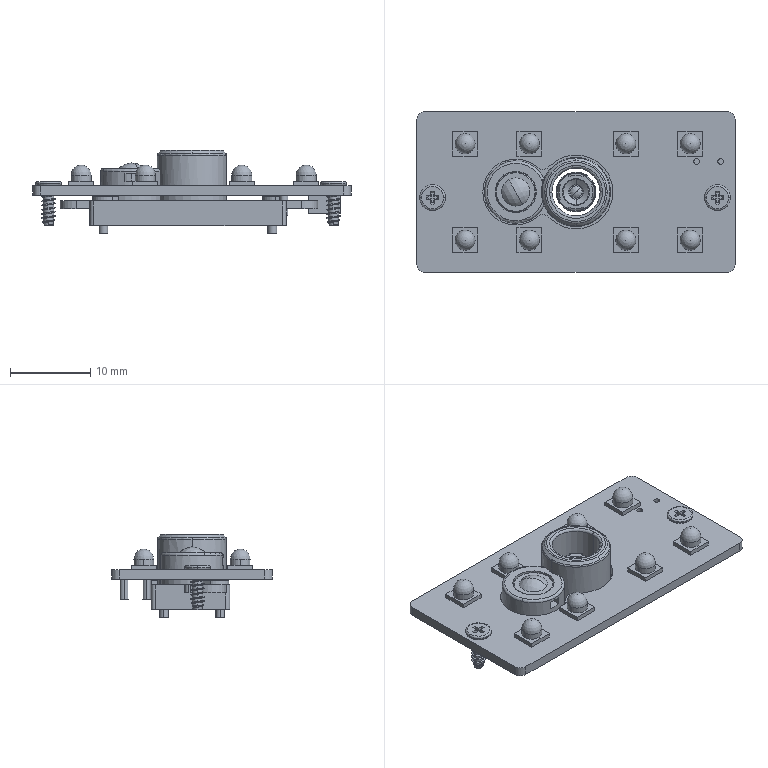Part | SolidWorks | 6 solids | 432 faces | box 39.6 x 20 x 10.4 mm | volume 1839 mm3 | cylinder 169 | plane 160 | cone 52 | torus 21 | spline 20 | sphere 10 | commonest cylinder face diameters 1.3 x38 2.5 x16 4.957 x15 4.74 x11 0.1 x8 1 x8